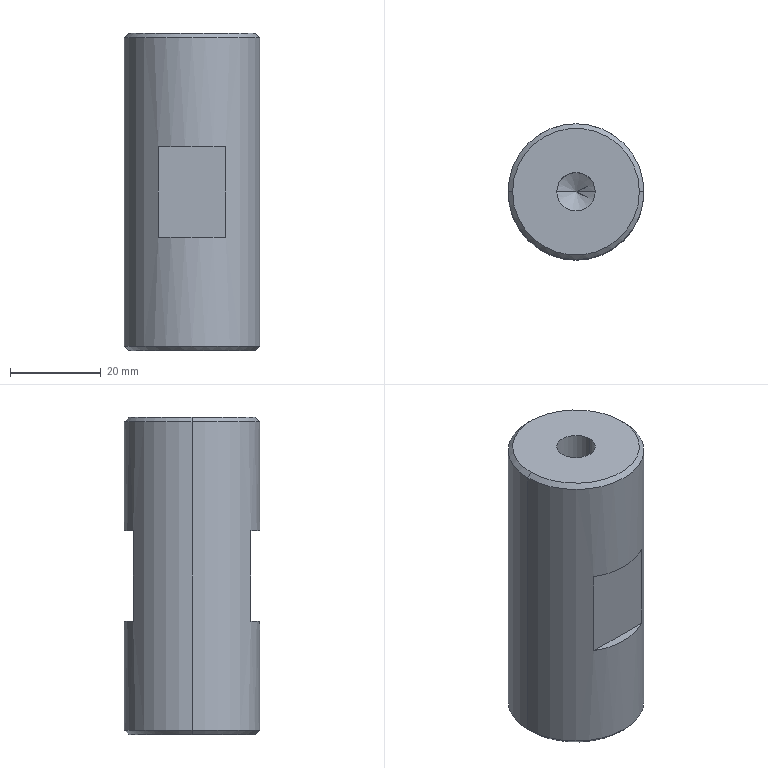Part | STEP file | BB013A02M-04-38A | 1 solid | 22 faces | box 30 x 30 x 70 mm | volume 45701 mm3 | cone 8 | plane 8 | cylinder 6 | commonest cylinder face diameters 8.5 x4 30 x2
STEP:
#1=CARTESIAN_POINT('',(0.,0.,0.));
#2=DIRECTION('',(0.,0.,1.));
#3=DIRECTION('',(1.,0.,0.));
#4=AXIS2_PLACEMENT_3D('',#1,#2,#3);
#5=CARTESIAN_POINT('',(7.483,13.,25.));
#6=VERTEX_POINT('',#5);
#7=CARTESIAN_POINT('',(7.483,13.,45.));
#8=VERTEX_POINT('',#7);
#9=CARTESIAN_POINT('',(7.483,13.,70.));
#10=DIRECTION('',(0.,0.,1.));
#11=VECTOR('',#10,1.);
#12=LINE('',#9,#11);
#13=CARTESIAN_POINT('',(0.,0.,70.));
#14=DIRECTION('',(0.,0.,-1.));
#15=DIRECTION('',(-1.,0.,0.));
#16=AXIS2_PLACEMENT_3D('',#13,#14,#15);
#17=CYLINDRICAL_SURFACE('',#16,15.);
#18=CARTESIAN_POINT('',(2.093,0.));
#19=DIRECTION('',(0.,-1.));
#20=VECTOR('',#19,1.);
#21=LINE('',#18,#20);
#22=(GEOMETRIC_REPRESENTATION_CONTEXT(2)PARAMETRIC_REPRESENTATION_CONTEXT()REPRESENTATION_CONTEXT('',''));
#23=DEFINITIONAL_REPRESENTATION('',(#21),#22);
#24=PCURVE('',#17,#23);
#25=CARTESIAN_POINT('',(7.483,13.,25.));
#26=DIRECTION('',(0.,1.,0.));
#27=DIRECTION('',(-1.,0.,0.));
#28=AXIS2_PLACEMENT_3D('',#25,#26,#27);
#29=PLANE('',#28);
#30=CARTESIAN_POINT('',(0.,45.));
#31=DIRECTION('',(0.,1.));
#32=VECTOR('',#31,1.);
#33=LINE('',#30,#32);
#34=(GEOMETRIC_REPRESENTATION_CONTEXT(2)PARAMETRIC_REPRESENTATION_CONTEXT()REPRESENTATION_CONTEXT('',''));
#35=DEFINITIONAL_REPRESENTATION('',(#33),#34);
#36=PCURVE('',#29,#35);
#37=SURFACE_CURVE('',#12,(#24,#36),.PCURVE_S1.);
#38=EDGE_CURVE('',#6,#8,#37,.T.);
#39=ORIENTED_EDGE('',*,*,#38,.T.);
#40=CARTESIAN_POINT('',(-7.483,13.,45.));
#41=VERTEX_POINT('',#40);
#42=CARTESIAN_POINT('',(0.,0.,45.));
#43=DIRECTION('',(0.,0.,1.));
#44=DIRECTION('',(-1.,0.,0.));
#45=AXIS2_PLACEMENT_3D('',#42,#43,#44);
#46=CIRCLE('',#45,15.);
#47=CARTESIAN_POINT('',(6.283,25.));
#48=DIRECTION('',(-1.,0.));
#49=VECTOR('',#48,1.);
#50=LINE('',#47,#49);
#51=(GEOMETRIC_REPRESENTATION_CONTEXT(2)PARAMETRIC_REPRESENTATION_CONTEXT()REPRESENTATION_CONTEXT('',''));
#52=DEFINITIONAL_REPRESENTATION('',(#50),#51);
#53=PCURVE('',#17,#52);
#54=CARTESIAN_POINT('',(0.,0.,45.));
#55=DIRECTION('',(0.,0.,-1.));
#56=DIRECTION('',(-1.,0.,0.));
#57=AXIS2_PLACEMENT_3D('',#54,#55,#56);
#58=PLANE('',#57);
#59=CARTESIAN_POINT('',(15.,0.));
#60=CARTESIAN_POINT('',(15.,-25.981));
#61=CARTESIAN_POINT('',(-7.5,-12.99));
#62=CARTESIAN_POINT('',(-30.,0.));
#63=CARTESIAN_POINT('',(-7.5,12.99));
#64=CARTESIAN_POINT('',(15.,25.981));
#65=CARTESIAN_POINT('',(15.,0.));
#66=(BOUNDED_CURVE()B_SPLINE_CURVE(2,(#59,#60,#61,#62,#63,#64,#65),.UNSPECIFIED.,.T.,.F.)B_SPLINE_CURVE_WITH_KNOTS((1,2,2,2,2,1),(-2.094,0.,2.094,4.189,6.283,8.378),.UNSPECIFIED.)CURVE()GEOMETRIC_REPRESENTATION_ITEM()RATIONAL_B_SPLINE_CURVE((1.,0.5,1.,0.5,1.,0.5,1.))REPRESENTATION_ITEM(''));
#67=(GEOMETRIC_REPRESENTATION_CONTEXT(2)PARAMETRIC_REPRESENTATION_CONTEXT()REPRESENTATION_CONTEXT('',''));
#68=DEFINITIONAL_REPRESENTATION('',(#66),#67);
#69=PCURVE('',#58,#68);
#70=SURFACE_CURVE('',#46,(#53,#69),.PCURVE_S1.);
#71=EDGE_CURVE('',#8,#41,#70,.T.);
#72=ORIENTED_EDGE('',*,*,#71,.T.);
#73=CARTESIAN_POINT('',(-7.483,13.,25.));
#74=VERTEX_POINT('',#73);
#75=CARTESIAN_POINT('',(-7.483,13.,70.));
#76=DIRECTION('',(0.,0.,-1.));
#77=VECTOR('',#76,1.);
#78=LINE('',#75,#77);
#79=CARTESIAN_POINT('',(1.048,0.));
#80=DIRECTION('',(0.,1.));
#81=VECTOR('',#80,1.);
#82=LINE('',#79,#81);
#83=(GEOMETRIC_REPRESENTATION_CONTEXT(2)PARAMETRIC_REPRESENTATION_CONTEXT()REPRESENTATION_CONTEXT('',''));
#84=DEFINITIONAL_REPRESENTATION('',(#82),#83);
#85=PCURVE('',#17,#84);
#86=CARTESIAN_POINT('',(14.967,45.));
#87=DIRECTION('',(0.,-1.));
#88=VECTOR('',#87,1.);
#89=LINE('',#86,#88);
#90=(GEOMETRIC_REPRESENTATION_CONTEXT(2)PARAMETRIC_REPRESENTATION_CONTEXT()REPRESENTATION_CONTEXT('',''));
#91=DEFINITIONAL_REPRESENTATION('',(#89),#90);
#92=PCURVE('',#29,#91);
#93=SURFACE_CURVE('',#78,(#85,#92),.PCURVE_S1.);
#94=EDGE_CURVE('',#41,#74,#93,.T.);
#95=ORIENTED_EDGE('',*,*,#94,.T.);
#96=CARTESIAN_POINT('',(0.,0.,25.));
#97=DIRECTION('',(0.,0.,-1.));
#98=DIRECTION('',(-1.,0.,0.));
#99=AXIS2_PLACEMENT_3D('',#96,#97,#98);
#100=CIRCLE('',#99,15.);
#101=CARTESIAN_POINT('',(0.,45.));
#102=DIRECTION('',(1.,0.));
#103=VECTOR('',#102,1.);
#104=LINE('',#101,#103);
#105=(GEOMETRIC_REPRESENTATION_CONTEXT(2)PARAMETRIC_REPRESENTATION_CONTEXT()REPRESENTATION_CONTEXT('',''));
#106=DEFINITIONAL_REPRESENTATION('',(#104),#105);
#107=PCURVE('',#17,#106);
#108=CARTESIAN_POINT('',(0.,0.,25.));
#109=DIRECTION('',(0.,0.,-1.));
#110=DIRECTION('',(-1.,0.,0.));
#111=AXIS2_PLACEMENT_3D('',#108,#109,#110);
#112=PLANE('',#111);
#113=CARTESIAN_POINT('',(0.,0.));
#114=DIRECTION('',(1.,0.));
#115=AXIS2_PLACEMENT_2D('',#113,#114);
#116=CIRCLE('',#115,15.);
#117=(GEOMETRIC_REPRESENTATION_CONTEXT(2)PARAMETRIC_REPRESENTATION_CONTEXT()REPRESENTATION_CONTEXT('',''));
#118=DEFINITIONAL_REPRESENTATION('',(#116),#117);
#119=PCURVE('',#112,#118);
#120=SURFACE_CURVE('',#100,(#107,#119),.PCURVE_S1.);
#121=EDGE_CURVE('',#74,#6,#120,.T.);
#122=ORIENTED_EDGE('',*,*,#121,.T.);
#123=EDGE_LOOP('',(#39,#72,#95,#122));
#124=FACE_BOUND('',#123,.T.);
#125=CARTESIAN_POINT('',(-15.,0.,69.));
#126=VERTEX_POINT('',#125);
#127=CARTESIAN_POINT('',(15.,0.,69.));
#128=VERTEX_POINT('',#127);
#129=CARTESIAN_POINT('',(0.,0.,69.));
#130=DIRECTION('',(0.,0.,-1.));
#131=DIRECTION('',(-1.,0.,0.));
#132=AXIS2_PLACEMENT_3D('',#129,#130,#131);
#133=CIRCLE('',#132,15.);
#134=CARTESIAN_POINT('',(0.,1.));
#135=DIRECTION('',(1.,0.));
#136=VECTOR('',#135,1.);
#137=LINE('',#134,#136);
#138=(GEOMETRIC_REPRESENTATION_CONTEXT(2)PARAMETRIC_REPRESENTATION_CONTEXT()REPRESENTATION_CONTEXT('',''));
#139=DEFINITIONAL_REPRESENTATION('',(#137),#138);
#140=PCURVE('',#17,#139);
#141=CARTESIAN_POINT('',(0.,0.,69.));
#142=DIRECTION('',(0.,0.,-1.));
#143=DIRECTION('',(-1.,0.,0.));
#144=AXIS2_PLACEMENT_3D('',#141,#142,#143);
#145=CONICAL_SURFACE('',#144,15.,0.7854);
#146=CARTESIAN_POINT('',(0.,0.));
#147=DIRECTION('',(1.,0.));
#148=VECTOR('',#147,1.);
#149=LINE('',#146,#148);
#150=(GEOMETRIC_REPRESENTATION_CONTEXT(2)PARAMETRIC_REPRESENTATION_CONTEXT()REPRESENTATION_CONTEXT('',''));
#151=DEFINITIONAL_REPRESENTATION('',(#149),#150);
#152=PCURVE('',#145,#151);
#153=SURFACE_CURVE('',#133,(#140,#152),.PCURVE_S1.);
#154=EDGE_CURVE('',#126,#128,#153,.T.);
#155=ORIENTED_EDGE('',*,*,#154,.T.);
#156=CARTESIAN_POINT('',(15.,0.,1.));
#157=VERTEX_POINT('',#156);
#158=CARTESIAN_POINT('',(15.,0.,70.));
#159=DIRECTION('',(0.,0.,-1.));
#160=VECTOR('',#159,1.);
#161=LINE('',#158,#160);
#162=CARTESIAN_POINT('',(3.142,0.));
#163=DIRECTION('',(0.,1.));
#164=VECTOR('',#163,1.);
#165=LINE('',#162,#164);
#166=(GEOMETRIC_REPRESENTATION_CONTEXT(2)PARAMETRIC_REPRESENTATION_CONTEXT()REPRESENTATION_CONTEXT('',''));
#167=DEFINITIONAL_REPRESENTATION('',(#165),#166);
#168=PCURVE('',#17,#167);
#169=CARTESIAN_POINT('',(0.,0.,70.));
#170=DIRECTION('',(0.,0.,-1.));
#171=DIRECTION('',(-1.,0.,0.));
#172=AXIS2_PLACEMENT_3D('',#169,#170,#171);
#173=CYLINDRICAL_SURFACE('',#172,15.);
#174=CARTESIAN_POINT('',(3.142,0.));
#175=DIRECTION('',(0.,1.));
#176=VECTOR('',#175,1.);
#177=LINE('',#174,#176);
#178=(GEOMETRIC_REPRESENTATION_CONTEXT(2)PARAMETRIC_REPRESENTATION_CONTEXT()REPRESENTATION_CONTEXT('',''));
#179=DEFINITIONAL_REPRESENTATION('',(#177),#178);
#180=PCURVE('',#173,#179);
#181=SURFACE_CURVE('',#161,(#168,#180),.PCURVE_S1.);
#182=EDGE_CURVE('',#128,#157,#181,.T.);
#183=ORIENTED_EDGE('',*,*,#182,.T.);
#184=CARTESIAN_POINT('',(-15.,0.,1.));
#185=VERTEX_POINT('',#184);
#186=CARTESIAN_POINT('',(0.,0.,1.));
#187=DIRECTION('',(0.,0.,1.));
#188=DIRECTION('',(-1.,0.,0.));
#189=AXIS2_PLACEMENT_3D('',#186,#187,#188);
#190=CIRCLE('',#189,15.);
#191=CARTESIAN_POINT('',(6.283,69.));
#192=DIRECTION('',(-1.,0.));
#193=VECTOR('',#192,1.);
#194=LINE('',#191,#193);
#195=(GEOMETRIC_REPRESENTATION_CONTEXT(2)PARAMETRIC_REPRESENTATION_CONTEXT()REPRESENTATION_CONTEXT('',''));
#196=DEFINITIONAL_REPRESENTATION('',(#194),#195);
#197=PCURVE('',#17,#196);
#198=CARTESIAN_POINT('',(0.,0.,1.));
#199=DIRECTION('',(0.,0.,1.));
#200=DIRECTION('',(1.,0.,0.));
#201=AXIS2_PLACEMENT_3D('',#198,#199,#200);
#202=CONICAL_SURFACE('',#201,15.,0.7854);
#203=CARTESIAN_POINT('',(-3.142,0.));
#204=DIRECTION('',(1.,0.));
#205=VECTOR('',#204,1.);
#206=LINE('',#203,#205);
#207=(GEOMETRIC_REPRESENTATION_CONTEXT(2)PARAMETRIC_REPRESENTATION_CONTEXT()REPRESENTATION_CONTEXT('',''));
#208=DEFINITIONAL_REPRESENTATION('',(#206),#207);
#209=PCURVE('',#202,#208);
#210=SURFACE_CURVE('',#190,(#197,#209),.PCURVE_S1.);
#211=EDGE_CURVE('',#157,#185,#210,.T.);
#212=ORIENTED_EDGE('',*,*,#211,.T.);
#213=CARTESIAN_POINT('',(-15.,0.,70.));
#214=DIRECTION('',(0.,0.,-1.));
#215=VECTOR('',#214,1.);
#216=LINE('',#213,#215);
#217=CARTESIAN_POINT('',(0.,0.));
#218=DIRECTION('',(0.,1.));
#219=VECTOR('',#218,1.);
#220=LINE('',#217,#219);
#221=(GEOMETRIC_REPRESENTATION_CONTEXT(2)PARAMETRIC_REPRESENTATION_CONTEXT()REPRESENTATION_CONTEXT('',''));
#222=DEFINITIONAL_REPRESENTATION('',(#220),#221);
#223=PCURVE('',#17,#222);
#224=CARTESIAN_POINT('',(6.283,0.));
#225=DIRECTION('',(0.,1.));
#226=VECTOR('',#225,1.);
#227=LINE('',#224,#226);
#228=(GEOMETRIC_REPRESENTATION_CONTEXT(2)PARAMETRIC_REPRESENTATION_CONTEXT()REPRESENTATION_CONTEXT('',''));
#229=DEFINITIONAL_REPRESENTATION('',(#227),#228);
#230=PCURVE('',#173,#229);
#231=SURFACE_CURVE('',#216,(#223,#230),.PCURVE_S1.);
#232=EDGE_CURVE('',#126,#185,#231,.T.);
#233=ORIENTED_EDGE('',*,*,#232,.F.);
#234=EDGE_LOOP('',(#155,#183,#212,#233));
#235=FACE_BOUND('',#234,.T.);
#236=ADVANCED_FACE('',(#124,#235),#17,.T.);
#237=CARTESIAN_POINT('',(14.,0.,0.));
#238=VERTEX_POINT('',#237);
#239=CARTESIAN_POINT('',(-14.,0.,0.));
#240=VERTEX_POINT('',#239);
#241=CARTESIAN_POINT('',(0.,0.,0.));
#242=DIRECTION('',(0.,0.,1.));
#243=DIRECTION('',(1.,0.,0.));
#244=AXIS2_PLACEMENT_3D('',#241,#242,#243);
#245=CIRCLE('',#244,14.);
#246=CARTESIAN_POINT('',(0.,-1.));
#247=DIRECTION('',(1.,0.));
#248=VECTOR('',#247,1.);
#249=LINE('',#246,#248);
#250=(GEOMETRIC_REPRESENTATION_CONTEXT(2)PARAMETRIC_REPRESENTATION_CONTEXT()REPRESENTATION_CONTEXT('',''));
#251=DEFINITIONAL_REPRESENTATION('',(#249),#250);
#252=PCURVE('',#202,#251);
#253=CARTESIAN_POINT('',(0.,0.,0.));
#254=DIRECTION('',(0.,0.,1.));
#255=DIRECTION('',(1.,0.,0.));
#256=AXIS2_PLACEMENT_3D('',#253,#254,#255);
#257=PLANE('',#256);
#258=CARTESIAN_POINT('',(0.,0.));
#259=DIRECTION('',(1.,0.));
#260=AXIS2_PLACEMENT_2D('',#258,#259);
#261=CIRCLE('',#260,14.);
#262=(GEOMETRIC_REPRESENTATION_CONTEXT(2)PARAMETRIC_REPRESENTATION_CONTEXT()REPRESENTATION_CONTEXT('',''));
#263=DEFINITIONAL_REPRESENTATION('',(#261),#262);
#264=PCURVE('',#257,#263);
#265=SURFACE_CURVE('',#245,(#252,#264),.PCURVE_S1.);
#266=EDGE_CURVE('',#238,#240,#265,.T.);
#267=ORIENTED_EDGE('',*,*,#266,.T.);
#268=CARTESIAN_POINT('',(-15.,0.,1.));
#269=DIRECTION('',(-0.7071,0.,0.7071));
#270=VECTOR('',#269,1.);
#271=LINE('',#268,#270);
#272=CARTESIAN_POINT('',(3.142,0.));
#273=DIRECTION('',(0.,1.));
#274=VECTOR('',#273,1.);
#275=LINE('',#272,#274);
#276=(GEOMETRIC_REPRESENTATION_CONTEXT(2)PARAMETRIC_REPRESENTATION_CONTEXT()REPRESENTATION_CONTEXT('',''));
#277=DEFINITIONAL_REPRESENTATION('',(#275),#276);
#278=PCURVE('',#202,#277);
#279=CARTESIAN_POINT('',(0.,0.,1.));
#280=DIRECTION('',(0.,0.,1.));
#281=DIRECTION('',(1.,0.,0.));
#282=AXIS2_PLACEMENT_3D('',#279,#280,#281);
#283=CONICAL_SURFACE('',#282,15.,0.7854);
#284=CARTESIAN_POINT('',(3.142,0.));
#285=DIRECTION('',(0.,1.));
#286=VECTOR('',#285,1.);
#287=LINE('',#284,#286);
#288=(GEOMETRIC_REPRESENTATION_CONTEXT(2)PARAMETRIC_REPRESENTATION_CONTEXT()REPRESENTATION_CONTEXT('',''));
#289=DEFINITIONAL_REPRESENTATION('',(#287),#288);
#290=PCURVE('',#283,#289);
#291=SURFACE_CURVE('',#271,(#278,#290),.PCURVE_S1.);
#292=EDGE_CURVE('',#240,#185,#291,.T.);
#293=ORIENTED_EDGE('',*,*,#292,.T.);
#294=ORIENTED_EDGE('',*,*,#211,.F.);
#295=CARTESIAN_POINT('',(15.,0.,1.));
#296=DIRECTION('',(0.7071,0.,0.7071));
#297=VECTOR('',#296,1.);
#298=LINE('',#295,#297);
#299=CARTESIAN_POINT('',(0.,0.));
#300=DIRECTION('',(0.,1.));
#301=VECTOR('',#300,1.);
#302=LINE('',#299,#301);
#303=(GEOMETRIC_REPRESENTATION_CONTEXT(2)PARAMETRIC_REPRESENTATION_CONTEXT()REPRESENTATION_CONTEXT('',''));
#304=DEFINITIONAL_REPRESENTATION('',(#302),#303);
#305=PCURVE('',#202,#304);
#306=CARTESIAN_POINT('',(6.283,0.));
#307=DIRECTION('',(0.,1.));
#308=VECTOR('',#307,1.);
#309=LINE('',#306,#308);
#310=(GEOMETRIC_REPRESENTATION_CONTEXT(2)PARAMETRIC_REPRESENTATION_CONTEXT()REPRESENTATION_CONTEXT('',''));
#311=DEFINITIONAL_REPRESENTATION('',(#309),#310);
#312=PCURVE('',#283,#311);
#313=SURFACE_CURVE('',#298,(#305,#312),.PCURVE_S1.);
#314=EDGE_CURVE('',#238,#157,#313,.T.);
#315=ORIENTED_EDGE('',*,*,#314,.F.);
#316=EDGE_LOOP('',(#267,#293,#294,#315));
#317=FACE_BOUND('',#316,.T.);
#318=ADVANCED_FACE('',(#317),#202,.T.);
#319=CARTESIAN_POINT('',(-14.,0.,70.));
#320=VERTEX_POINT('',#319);
#321=CARTESIAN_POINT('',(14.,0.,70.));
#322=VERTEX_POINT('',#321);
#323=CARTESIAN_POINT('',(0.,0.,70.));
#324=DIRECTION('',(0.,0.,-1.));
#325=DIRECTION('',(-1.,0.,0.));
#326=AXIS2_PLACEMENT_3D('',#323,#324,#325);
#327=CIRCLE('',#326,14.);
#328=CARTESIAN_POINT('',(0.,-1.));
#329=DIRECTION('',(1.,0.));
#330=VECTOR('',#329,1.);
#331=LINE('',#328,#330);
#332=(GEOMETRIC_REPRESENTATION_CONTEXT(2)PARAMETRIC_REPRESENTATION_CONTEXT()REPRESENTATION_CONTEXT('',''));
#333=DEFINITIONAL_REPRESENTATION('',(#331),#332);
#334=PCURVE('',#145,#333);
#335=CARTESIAN_POINT('',(0.,0.,70.));
#336=DIRECTION('',(0.,0.,1.));
#337=DIRECTION('',(1.,0.,0.));
#338=AXIS2_PLACEMENT_3D('',#335,#336,#337);
#339=PLANE('',#338);
#340=CARTESIAN_POINT('',(-14.,0.));
#341=CARTESIAN_POINT('',(-14.,24.249));
#342=CARTESIAN_POINT('',(7.,12.124));
#343=CARTESIAN_POINT('',(28.,0.));
#344=CARTESIAN_POINT('',(7.,-12.124));
#345=CARTESIAN_POINT('',(-14.,-24.249));
#346=CARTESIAN_POINT('',(-14.,0.));
#347=(BOUNDED_CURVE()B_SPLINE_CURVE(2,(#340,#341,#342,#343,#344,#345,#346),.UNSPECIFIED.,.T.,.F.)B_SPLINE_CURVE_WITH_KNOTS((1,2,2,2,2,1),(-2.094,0.,2.094,4.189,6.283,8.378),.UNSPECIFIED.)CURVE()GEOMETRIC_REPRESENTATION_ITEM()RATIONAL_B_SPLINE_CURVE((1.,0.5,1.,0.5,1.,0.5,1.))REPRESENTATION_ITEM(''));
#348=(GEOMETRIC_REPRESENTATION_CONTEXT(2)PARAMETRIC_REPRESENTATION_CONTEXT()REPRESENTATION_CONTEXT('',''));
#349=DEFINITIONAL_REPRESENTATION('',(#347),#348);
#350=PCURVE('',#339,#349);
#351=SURFACE_CURVE('',#327,(#334,#350),.PCURVE_S1.);
#352=EDGE_CURVE('',#320,#322,#351,.T.);
#353=ORIENTED_EDGE('',*,*,#352,.T.);
#354=CARTESIAN_POINT('',(15.,0.,69.));
#355=DIRECTION('',(0.7071,0.,-0.7071));
#356=VECTOR('',#355,1.);
#357=LINE('',#354,#356);
#358=CARTESIAN_POINT('',(3.142,0.));
#359=DIRECTION('',(0.,1.));
#360=VECTOR('',#359,1.);
#361=LINE('',#358,#360);
#362=(GEOMETRIC_REPRESENTATION_CONTEXT(2)PARAMETRIC_REPRESENTATION_CONTEXT()REPRESENTATION_CONTEXT('',''));
#363=DEFINITIONAL_REPRESENTATION('',(#361),#362);
#364=PCURVE('',#145,#363);
#365=CARTESIAN_POINT('',(0.,0.,69.));
#366=DIRECTION('',(0.,0.,-1.));
#367=DIRECTION('',(-1.,0.,0.));
#368=AXIS2_PLACEMENT_3D('',#365,#366,#367);
#369=CONICAL_SURFACE('',#368,15.,0.7854);
#370=CARTESIAN_POINT('',(3.142,0.));
#371=DIRECTION('',(0.,1.));
#372=VECTOR('',#371,1.);
#373=LINE('',#370,#372);
#374=(GEOMETRIC_REPRESENTATION_CONTEXT(2)PARAMETRIC_REPRESENTATION_CONTEXT()REPRESENTATION_CONTEXT('',''));
#375=DEFINITIONAL_REPRESENTATION('',(#373),#374);
#376=PCURVE('',#369,#375);
#377=SURFACE_CURVE('',#357,(#364,#376),.PCURVE_S1.);
#378=EDGE_CURVE('',#322,#128,#377,.T.);
#379=ORIENTED_EDGE('',*,*,#378,.T.);
#380=ORIENTED_EDGE('',*,*,#154,.F.);
#381=CARTESIAN_POINT('',(-15.,0.,69.));
#382=DIRECTION('',(-0.7071,0.,-0.7071));
#383=VECTOR('',#382,1.);
#384=LINE('',#381,#383);
#385=CARTESIAN_POINT('',(0.,0.));
#386=DIRECTION('',(0.,1.));
#387=VECTOR('',#386,1.);
#388=LINE('',#385,#387);
#389=(GEOMETRIC_REPRESENTATION_CONTEXT(2)PARAMETRIC_REPRESENTATION_CONTEXT()REPRESENTATION_CONTEXT('',''));
#390=DEFINITIONAL_REPRESENTATION('',(#388),#389);
#391=PCURVE('',#145,#390);
#392=CARTESIAN_POINT('',(6.283,0.));
#393=DIRECTION('',(0.,1.));
#394=VECTOR('',#393,1.);
#395=LINE('',#392,#394);
#396=(GEOMETRIC_REPRESENTATION_CONTEXT(2)PARAMETRIC_REPRESENTATION_CONTEXT()REPRESENTATION_CONTEXT('',''));
#397=DEFINITIONAL_REPRESENTATION('',(#395),#396);
#398=PCURVE('',#369,#397);
#399=SURFACE_CURVE('',#384,(#391,#398),.PCURVE_S1.);
#400=EDGE_CURVE('',#320,#126,#399,.T.);
#401=ORIENTED_EDGE('',*,*,#400,.F.);
#402=EDGE_LOOP('',(#353,#379,#380,#401));
#403=FACE_BOUND('',#402,.T.);
#404=ADVANCED_FACE('',(#403),#145,.T.);
#405=CARTESIAN_POINT('',(-4.25,0.,24.5));
#406=VERTEX_POINT('',#405);
#407=CARTESIAN_POINT('',(-4.25,0.,0.));
#408=VERTEX_POINT('',#407);
#409=CARTESIAN_POINT('',(-4.25,0.,0.));
#410=DIRECTION('',(0.,0.,-1.));
#411=VECTOR('',#410,1.);
#412=LINE('',#409,#411);
#413=CARTESIAN_POINT('',(0.,0.,0.));
#414=DIRECTION('',(0.,0.,-1.));
#415=DIRECTION('',(-1.,0.,0.));
#416=AXIS2_PLACEMENT_3D('',#413,#414,#415);
#417=CYLINDRICAL_SURFACE('',#416,4.25);
#418=CARTESIAN_POINT('',(6.283,0.));
#419=DIRECTION('',(0.,1.));
#420=VECTOR('',#419,1.);
#421=LINE('',#418,#420);
#422=(GEOMETRIC_REPRESENTATION_CONTEXT(2)PARAMETRIC_REPRESENTATION_CONTEXT()REPRESENTATION_CONTEXT('',''));
#423=DEFINITIONAL_REPRESENTATION('',(#421),#422);
#424=PCURVE('',#417,#423);
#425=CARTESIAN_POINT('',(0.,0.,0.));
#426=DIRECTION('',(0.,0.,-1.));
#427=DIRECTION('',(-1.,0.,0.));
#428=AXIS2_PLACEMENT_3D('',#425,#426,#427);
#429=CYLINDRICAL_SURFACE('',#428,4.25);
#430=CARTESIAN_POINT('',(0.,0.));
#431=DIRECTION('',(0.,1.));
#432=VECTOR('',#431,1.);
#433=LINE('',#430,#432);
#434=(GEOMETRIC_REPRESENTATION_CONTEXT(2)PARAMETRIC_REPRESENTATION_CONTEXT()REPRESENTATION_CONTEXT('',''));
#435=DEFINITIONAL_REPRESENTATION('',(#433),#434);
#436=PCURVE('',#429,#435);
#437=SURFACE_CURVE('',#412,(#424,#436),.PCURVE_S1.);
#438=EDGE_CURVE('',#406,#408,#437,.T.);
#439=ORIENTED_EDGE('',*,*,#438,.T.);
#440=CARTESIAN_POINT('',(4.25,0.,0.));
#441=VERTEX_POINT('',#440);
#442=CARTESIAN_POINT('',(0.,0.,0.));
#443=DIRECTION('',(0.,0.,-1.));
#444=DIRECTION('',(-1.,0.,0.));
#445=AXIS2_PLACEMENT_3D('',#442,#443,#444);
#446=CIRCLE('',#445,4.25);
#447=CARTESIAN_POINT('',(0.,0.));
#448=DIRECTION('',(1.,0.));
#449=VECTOR('',#448,1.);
#450=LINE('',#447,#449);
#451=(GEOMETRIC_REPRESENTATION_CONTEXT(2)PARAMETRIC_REPRESENTATION_CONTEXT()REPRESENTATION_CONTEXT('',''));
#452=DEFINITIONAL_REPRESENTATION('',(#450),#451);
#453=PCURVE('',#417,#452);
#454=CARTESIAN_POINT('',(-4.25,0.));
#455=CARTESIAN_POINT('',(-4.25,7.361));
#456=CARTESIAN_POINT('',(2.125,3.681));
#457=CARTESIAN_POINT('',(8.5,0.));
#458=CARTESIAN_POINT('',(2.125,-3.681));
#459=CARTESIAN_POINT('',(-4.25,-7.361));
#460=CARTESIAN_POINT('',(-4.25,0.));
#461=(BOUNDED_CURVE()B_SPLINE_CURVE(2,(#454,#455,#456,#457,#458,#459,#460),.UNSPECIFIED.,.T.,.F.)B_SPLINE_CURVE_WITH_KNOTS((1,2,2,2,2,1),(-2.094,0.,2.094,4.189,6.283,8.378),.UNSPECIFIED.)CURVE()GEOMETRIC_REPRESENTATION_ITEM()RATIONAL_B_SPLINE_CURVE((1.,0.5,1.,0.5,1.,0.5,1.))REPRESENTATION_ITEM(''));
#462=(GEOMETRIC_REPRESENTATION_CONTEXT(2)PARAMETRIC_REPRESENTATION_CONTEXT()REPRESENTATION_CONTEXT('',''));
#463=DEFINITIONAL_REPRESENTATION('',(#461),#462);
#464=PCURVE('',#257,#463);
#465=SURFACE_CURVE('',#446,(#453,#464),.PCURVE_S1.);
#466=EDGE_CURVE('',#441,#408,#465,.T.);
#467=ORIENTED_EDGE('',*,*,#466,.F.);
#468=CARTESIAN_POINT('',(4.25,0.,24.5));
#469=VERTEX_POINT('',#468);
#470=CARTESIAN_POINT('',(4.25,0.,0.));
#471=DIRECTION('',(0.,0.,-1.));
#472=VECTOR('',#471,1.);
#473=LINE('',#470,#472);
#474=CARTESIAN_POINT('',(3.142,0.));
#475=DIRECTION('',(0.,1.));
#476=VECTOR('',#475,1.);
#477=LINE('',#474,#476);
#478=(GEOMETRIC_REPRESENTATION_CONTEXT(2)PARAMETRIC_REPRESENTATION_CONTEXT()REPRESENTATION_CONTEXT('',''));
#479=DEFINITIONAL_REPRESENTATION('',(#477),#478);
#480=PCURVE('',#417,#479);
#481=CARTESIAN_POINT('',(3.142,0.));
#482=DIRECTION('',(0.,1.));
#483=VECTOR('',#482,1.);
#484=LINE('',#481,#483);
#485=(GEOMETRIC_REPRESENTATION_CONTEXT(2)PARAMETRIC_REPRESENTATION_CONTEXT()REPRESENTATION_CONTEXT('',''));
#486=DEFINITIONAL_REPRESENTATION('',(#484),#485);
#487=PCURVE('',#429,#486);
#488=SURFACE_CURVE('',#473,(#480,#487),.PCURVE_S1.);
#489=EDGE_CURVE('',#469,#441,#488,.T.);
#490=ORIENTED_EDGE('',*,*,#489,.F.);
#491=CARTESIAN_POINT('',(0.,0.,24.5));
#492=DIRECTION('',(0.,0.,-1.));
#493=DIRECTION('',(-1.,0.,0.));
#494=AXIS2_PLACEMENT_3D('',#491,#492,#493);
#495=CIRCLE('',#494,4.25);
#496=CARTESIAN_POINT('',(0.,-24.5));
#497=DIRECTION('',(1.,0.));
#498=VECTOR('',#497,1.);
#499=LINE('',#496,#498);
#500=(GEOMETRIC_REPRESENTATION_CONTEXT(2)PARAMETRIC_REPRESENTATION_CONTEXT()REPRESENTATION_CONTEXT('',''));
#501=DEFINITIONAL_REPRESENTATION('',(#499),#500);
#502=PCURVE('',#417,#501);
#503=CARTESIAN_POINT('',(0.,0.,24.5));
#504=DIRECTION('',(0.,0.,-1.));
#505=DIRECTION('',(-1.,0.,0.));
#506=AXIS2_PLACEMENT_3D('',#503,#504,#505);
#507=CONICAL_SURFACE('',#506,4.25,1.03);
#508=CARTESIAN_POINT('',(0.,0.));
#509=DIRECTION('',(1.,0.));
#510=VECTOR('',#509,1.);
#511=LINE('',#508,#510);
#512=(GEOMETRIC_REPRESENTATION_CONTEXT(2)PARAMETRIC_REPRESENTATION_CONTEXT()REPRESENTATION_CONTEXT('',''));
#513=DEFINITIONAL_REPRESENTATION('',(#511),#512);
#514=PCURVE('',#507,#513);
#515=SURFACE_CURVE('',#495,(#502,#514),.PCURVE_S1.);
#516=EDGE_CURVE('',#469,#406,#515,.T.);
#517=ORIENTED_EDGE('',*,*,#516,.T.);
#518=EDGE_LOOP('',(#439,#467,#490,#517));
#519=FACE_BOUND('',#518,.F.);
#520=ADVANCED_FACE('',(#519),#417,.F.);
#521=CARTESIAN_POINT('',(4.25,0.,45.5));
#522=VERTEX_POINT('',#521);
#523=CARTESIAN_POINT('',(4.25,0.,70.));
#524=VERTEX_POINT('',#523);
#525=CARTESIAN_POINT('',(4.25,0.,70.));
#526=DIRECTION('',(0.,0.,1.));
#527=VECTOR('',#526,1.);
#528=LINE('',#525,#527);
#529=CARTESIAN_POINT('',(0.,0.,70.));
#530=DIRECTION('',(0.,0.,1.));
#531=DIRECTION('',(1.,0.,0.));
#532=AXIS2_PLACEMENT_3D('',#529,#530,#531);
#533=CYLINDRICAL_SURFACE('',#532,4.25);
#534=CARTESIAN_POINT('',(6.283,0.));
#535=DIRECTION('',(0.,1.));
#536=VECTOR('',#535,1.);
#537=LINE('',#534,#536);
#538=(GEOMETRIC_REPRESENTATION_CONTEXT(2)PARAMETRIC_REPRESENTATION_CONTEXT()REPRESENTATION_CONTEXT('',''));
#539=DEFINITIONAL_REPRESENTATION('',(#537),#538);
#540=PCURVE('',#533,#539);
#541=CARTESIAN_POINT('',(0.,0.,70.));
#542=DIRECTION('',(0.,0.,1.));
#543=DIRECTION('',(1.,0.,0.));
#544=AXIS2_PLACEMENT_3D('',#541,#542,#543);
#545=CYLINDRICAL_SURFACE('',#544,4.25);
#546=CARTESIAN_POINT('',(0.,0.));
#547=DIRECTION('',(0.,1.));
#548=VECTOR('',#547,1.);
#549=LINE('',#546,#548);
#550=(GEOMETRIC_REPRESENTATION_CONTEXT(2)PARAMETRIC_REPRESENTATION_CONTEXT()REPRESENTATION_CONTEXT('',''));
#551=DEFINITIONAL_REPRESENTATION('',(#549),#550);
#552=PCURVE('',#545,#551);
#553=SURFACE_CURVE('',#528,(#540,#552),.PCURVE_S1.);
#554=EDGE_CURVE('',#522,#524,#553,.T.);
#555=ORIENTED_EDGE('',*,*,#554,.T.);
#556=CARTESIAN_POINT('',(-4.25,0.,70.));
#557=VERTEX_POINT('',#556);
#558=CARTESIAN_POINT('',(0.,0.,70.));
#559=DIRECTION('',(0.,0.,-1.));
#560=DIRECTION('',(1.,0.,0.));
#561=AXIS2_PLACEMENT_3D('',#558,#559,#560);
#562=CIRCLE('',#561,4.25);
#563=CARTESIAN_POINT('',(6.283,0.));
#564=DIRECTION('',(-1.,0.));
#565=VECTOR('',#564,1.);
#566=LINE('',#563,#565);
#567=(GEOMETRIC_REPRESENTATION_CONTEXT(2)PARAMETRIC_REPRESENTATION_CONTEXT()REPRESENTATION_CONTEXT('',''));
#568=DEFINITIONAL_REPRESENTATION('',(#566),#567);
#569=PCURVE('',#533,#568);
#570=CARTESIAN_POINT('',(4.25,0.));
#571=CARTESIAN_POINT('',(4.25,-7.361));
#572=CARTESIAN_POINT('',(-2.125,-3.681));
#573=CARTESIAN_POINT('',(-8.5,0.));
#574=CARTESIAN_POINT('',(-2.125,3.681));
#575=CARTESIAN_POINT('',(4.25,7.361));
#576=CARTESIAN_POINT('',(4.25,0.));
#577=(BOUNDED_CURVE()B_SPLINE_CURVE(2,(#570,#571,#572,#573,#574,#575,#576),.UNSPECIFIED.,.T.,.F.)B_SPLINE_CURVE_WITH_KNOTS((1,2,2,2,2,1),(-2.094,0.,2.094,4.189,6.283,8.378),.UNSPECIFIED.)CURVE()GEOMETRIC_REPRESENTATION_ITEM()RATIONAL_B_SPLINE_CURVE((1.,0.5,1.,0.5,1.,0.5,1.))REPRESENTATION_ITEM(''));
#578=(GEOMETRIC_REPRESENTATION_CONTEXT(2)PARAMETRIC_REPRESENTATION_CONTEXT()REPRESENTATION_CONTEXT('',''));
#579=DEFINITIONAL_REPRESENTATION('',(#577),#578);
#580=PCURVE('',#339,#579);
#581=SURFACE_CURVE('',#562,(#569,#580),.PCURVE_S1.);
#582=EDGE_CURVE('',#524,#557,#581,.T.);
#583=ORIENTED_EDGE('',*,*,#582,.T.);
#584=CARTESIAN_POINT('',(-4.25,0.,45.5));
#585=VERTEX_POINT('',#584);
#586=CARTESIAN_POINT('',(-4.25,0.,70.));
#587=DIRECTION('',(0.,0.,1.));
#588=VECTOR('',#587,1.);
#589=LINE('',#586,#588);
#590=CARTESIAN_POINT('',(3.142,0.));
#591=DIRECTION('',(0.,1.));
#592=VECTOR('',#591,1.);
#593=LINE('',#590,#592);
#594=(GEOMETRIC_REPRESENTATION_CONTEXT(2)PARAMETRIC_REPRESENTATION_CONTEXT()REPRESENTATION_CONTEXT('',''));
#595=DEFINITIONAL_REPRESENTATION('',(#593),#594);
#596=PCURVE('',#533,#595);
#597=CARTESIAN_POINT('',(3.142,0.));
#598=DIRECTION('',(0.,1.));
#599=VECTOR('',#598,1.);
#600=LINE('',#597,#599);
#601=(GEOMETRIC_REPRESENTATION_CONTEXT(2)PARAMETRIC_REPRESENTATION_CONTEXT()REPRESENTATION_CONTEXT('',''));
#602=DEFINITIONAL_REPRESENTATION('',(#600),#601);
#603=PCURVE('',#545,#602);
#604=SURFACE_CURVE('',#589,(#596,#603),.PCURVE_S1.);
#605=EDGE_CURVE('',#585,#557,#604,.T.);
#606=ORIENTED_EDGE('',*,*,#605,.F.);
#607=CARTESIAN_POINT('',(0.,0.,45.5));
#608=DIRECTION('',(0.,0.,1.));
#609=DIRECTION('',(1.,0.,0.));
#610=AXIS2_PLACEMENT_3D('',#607,#608,#609);
#611=CIRCLE('',#610,4.25);
#612=CARTESIAN_POINT('',(0.,-24.5));
#613=DIRECTION('',(1.,0.));
#614=VECTOR('',#613,1.);
#615=LINE('',#612,#614);
#616=(GEOMETRIC_REPRESENTATION_CONTEXT(2)PARAMETRIC_REPRESENTATION_CONTEXT()REPRESENTATION_CONTEXT('',''));
#617=DEFINITIONAL_REPRESENTATION('',(#615),#616);
#618=PCURVE('',#533,#617);
#619=CARTESIAN_POINT('',(0.,0.,45.5));
#620=DIRECTION('',(0.,0.,1.));
#621=DIRECTION('',(1.,0.,0.));
#622=AXIS2_PLACEMENT_3D('',#619,#620,#621);
#623=CONICAL_SURFACE('',#622,4.25,1.03);
#624=CARTESIAN_POINT('',(0.,0.));
#625=DIRECTION('',(1.,0.));
#626=VECTOR('',#625,1.);
#627=LINE('',#624,#626);
#628=(GEOMETRIC_REPRESENTATION_CONTEXT(2)PARAMETRIC_REPRESENTATION_CONTEXT()REPRESENTATION_CONTEXT('',''));
#629=DEFINITIONAL_REPRESENTATION('',(#627),#628);
#630=PCURVE('',#623,#629);
#631=SURFACE_CURVE('',#611,(#618,#630),.PCURVE_S1.);
#632=EDGE_CURVE('',#585,#522,#631,.T.);
#633=ORIENTED_EDGE('',*,*,#632,.T.);
#634=EDGE_LOOP('',(#555,#583,#606,#633));
#635=FACE_BOUND('',#634,.F.);
#636=ADVANCED_FACE('',(#635),#533,.F.);
#637=ORIENTED_EDGE('',*,*,#516,.F.);
#638=CARTESIAN_POINT('',(0.,0.,27.054));
#639=VERTEX_POINT('',#638);
#640=CARTESIAN_POINT('',(4.25,0.,24.5));
#641=DIRECTION('',(0.8572,0.,-0.515));
#642=VECTOR('',#641,1.);
#643=LINE('',#640,#642);
#644=CARTESIAN_POINT('',(3.142,0.));
#645=DIRECTION('',(0.,1.));
#646=VECTOR('',#645,1.);
#647=LINE('',#644,#646);
#648=(GEOMETRIC_REPRESENTATION_CONTEXT(2)PARAMETRIC_REPRESENTATION_CONTEXT()REPRESENTATION_CONTEXT('',''));
#649=DEFINITIONAL_REPRESENTATION('',(#647),#648);
#650=PCURVE('',#507,#649);
#651=CARTESIAN_POINT('',(0.,0.,24.5));
#652=DIRECTION('',(0.,0.,-1.));
#653=DIRECTION('',(-1.,0.,0.));
#654=AXIS2_PLACEMENT_3D('',#651,#652,#653);
#655=CONICAL_SURFACE('',#654,4.25,1.03);
#656=CARTESIAN_POINT('',(3.142,0.));
#657=DIRECTION('',(0.,1.));
#658=VECTOR('',#657,1.);
#659=LINE('',#656,#658);
#660=(GEOMETRIC_REPRESENTATION_CONTEXT(2)PARAMETRIC_REPRESENTATION_CONTEXT()REPRESENTATION_CONTEXT('',''));
#661=DEFINITIONAL_REPRESENTATION('',(#659),#660);
#662=PCURVE('',#655,#661);
#663=SURFACE_CURVE('',#643,(#650,#662),.PCURVE_S1.);
#664=EDGE_CURVE('',#639,#469,#663,.T.);
#665=ORIENTED_EDGE('',*,*,#664,.F.);
#666=CARTESIAN_POINT('',(-4.25,0.,24.5));
#667=DIRECTION('',(-0.8572,0.,-0.515));
#668=VECTOR('',#667,1.);
#669=LINE('',#666,#668);
#670=CARTESIAN_POINT('',(6.283,0.));
#671=DIRECTION('',(0.,1.));
#672=VECTOR('',#671,1.);
#673=LINE('',#670,#672);
#674=(GEOMETRIC_REPRESENTATION_CONTEXT(2)PARAMETRIC_REPRESENTATION_CONTEXT()REPRESENTATION_CONTEXT('',''));
#675=DEFINITIONAL_REPRESENTATION('',(#673),#674);
#676=PCURVE('',#507,#675);
#677=CARTESIAN_POINT('',(0.,0.));
#678=DIRECTION('',(0.,1.));
#679=VECTOR('',#678,1.);
#680=LINE('',#677,#679);
#681=(GEOMETRIC_REPRESENTATION_CONTEXT(2)PARAMETRIC_REPRESENTATION_CONTEXT()REPRESENTATION_CONTEXT('',''));
#682=DEFINITIONAL_REPRESENTATION('',(#680),#681);
#683=PCURVE('',#655,#682);
#684=SURFACE_CURVE('',#669,(#676,#683),.PCURVE_S1.);
#685=EDGE_CURVE('',#639,#406,#684,.T.);
#686=ORIENTED_EDGE('',*,*,#685,.T.);
#687=EDGE_LOOP('',(#637,#665,#686));
#688=FACE_BOUND('',#687,.F.);
#689=ADVANCED_FACE('',(#688),#507,.F.);
#690=ORIENTED_EDGE('',*,*,#632,.F.);
#691=CARTESIAN_POINT('',(0.,0.,42.946));
#692=VERTEX_POINT('',#691);
#693=CARTESIAN_POINT('',(-4.25,0.,45.5));
#694=DIRECTION('',(-0.8572,0.,0.515));
#695=VECTOR('',#694,1.);
#696=LINE('',#693,#695);
#697=CARTESIAN_POINT('',(3.142,0.));
#698=DIRECTION('',(0.,1.));
#699=VECTOR('',#698,1.);
#700=LINE('',#697,#699);
#701=(GEOMETRIC_REPRESENTATION_CONTEXT(2)PARAMETRIC_REPRESENTATION_CONTEXT()REPRESENTATION_CONTEXT('',''));
#702=DEFINITIONAL_REPRESENTATION('',(#700),#701);
#703=PCURVE('',#623,#702);
#704=CARTESIAN_POINT('',(0.,0.,45.5));
#705=DIRECTION('',(0.,0.,1.));
#706=DIRECTION('',(1.,0.,0.));
#707=AXIS2_PLACEMENT_3D('',#704,#705,#706);
#708=CONICAL_SURFACE('',#707,4.25,1.03);
#709=CARTESIAN_POINT('',(3.142,0.));
#710=DIRECTION('',(0.,1.));
#711=VECTOR('',#710,1.);
#712=LINE('',#709,#711);
#713=(GEOMETRIC_REPRESENTATION_CONTEXT(2)PARAMETRIC_REPRESENTATION_CONTEXT()REPRESENTATION_CONTEXT('',''));
#714=DEFINITIONAL_REPRESENTATION('',(#712),#713);
#715=PCURVE('',#708,#714);
#716=SURFACE_CURVE('',#696,(#703,#715),.PCURVE_S1.);
#717=EDGE_CURVE('',#692,#585,#716,.T.);
#718=ORIENTED_EDGE('',*,*,#717,.F.);
#719=CARTESIAN_POINT('',(4.25,0.,45.5));
#720=DIRECTION('',(0.8572,0.,0.515));
#721=VECTOR('',#720,1.);
#722=LINE('',#719,#721);
#723=CARTESIAN_POINT('',(6.283,0.));
#724=DIRECTION('',(0.,1.));
#725=VECTOR('',#724,1.);
#726=LINE('',#723,#725);
#727=(GEOMETRIC_REPRESENTATION_CONTEXT(2)PARAMETRIC_REPRESENTATION_CONTEXT()REPRESENTATION_CONTEXT('',''));
#728=DEFINITIONAL_REPRESENTATION('',(#726),#727);
#729=PCURVE('',#623,#728);
#730=CARTESIAN_POINT('',(0.,0.));
#731=DIRECTION('',(0.,1.));
#732=VECTOR('',#731,1.);
#733=LINE('',#730,#732);
#734=(GEOMETRIC_REPRESENTATION_CONTEXT(2)PARAMETRIC_REPRESENTATION_CONTEXT()REPRESENTATION_CONTEXT('',''));
#735=DEFINITIONAL_REPRESENTATION('',(#733),#734);
#736=PCURVE('',#708,#735);
#737=SURFACE_CURVE('',#722,(#729,#736),.PCURVE_S1.);
#738=EDGE_CURVE('',#692,#522,#737,.T.);
#739=ORIENTED_EDGE('',*,*,#738,.T.);
#740=EDGE_LOOP('',(#690,#718,#739));
#741=FACE_BOUND('',#740,.F.);
#742=ADVANCED_FACE('',(#741),#623,.F.);
#743=ORIENTED_EDGE('',*,*,#182,.F.);
#744=CARTESIAN_POINT('',(0.,0.,69.));
#745=DIRECTION('',(0.,0.,-1.));
#746=DIRECTION('',(-1.,0.,0.));
#747=AXIS2_PLACEMENT_3D('',#744,#745,#746);
#748=CIRCLE('',#747,15.);
#749=CARTESIAN_POINT('',(0.,1.));
#750=DIRECTION('',(1.,0.));
#751=VECTOR('',#750,1.);
#752=LINE('',#749,#751);
#753=(GEOMETRIC_REPRESENTATION_CONTEXT(2)PARAMETRIC_REPRESENTATION_CONTEXT()REPRESENTATION_CONTEXT('',''));
#754=DEFINITIONAL_REPRESENTATION('',(#752),#753);
#755=PCURVE('',#173,#754);
#756=CARTESIAN_POINT('',(0.,0.));
#757=DIRECTION('',(1.,0.));
#758=VECTOR('',#757,1.);
#759=LINE('',#756,#758);
#760=(GEOMETRIC_REPRESENTATION_CONTEXT(2)PARAMETRIC_REPRESENTATION_CONTEXT()REPRESENTATION_CONTEXT('',''));
#761=DEFINITIONAL_REPRESENTATION('',(#759),#760);
#762=PCURVE('',#369,#761);
#763=SURFACE_CURVE('',#748,(#755,#762),.PCURVE_S1.);
#764=EDGE_CURVE('',#128,#126,#763,.T.);
#765=ORIENTED_EDGE('',*,*,#764,.T.);
#766=ORIENTED_EDGE('',*,*,#232,.T.);
#767=CARTESIAN_POINT('',(0.,0.,1.));
#768=DIRECTION('',(0.,0.,1.));
#769=DIRECTION('',(-1.,0.,0.));
#770=AXIS2_PLACEMENT_3D('',#767,#768,#769);
#771=CIRCLE('',#770,15.);
#772=CARTESIAN_POINT('',(6.283,69.));
#773=DIRECTION('',(-1.,0.));
#774=VECTOR('',#773,1.);
#775=LINE('',#772,#774);
#776=(GEOMETRIC_REPRESENTATION_CONTEXT(2)PARAMETRIC_REPRESENTATION_CONTEXT()REPRESENTATION_CONTEXT('',''));
#777=DEFINITIONAL_REPRESENTATION('',(#775),#776);
#778=PCURVE('',#173,#777);
#779=CARTESIAN_POINT('',(3.142,0.));
#780=DIRECTION('',(1.,0.));
#781=VECTOR('',#780,1.);
#782=LINE('',#779,#781);
#783=(GEOMETRIC_REPRESENTATION_CONTEXT(2)PARAMETRIC_REPRESENTATION_CONTEXT()REPRESENTATION_CONTEXT('',''));
#784=DEFINITIONAL_REPRESENTATION('',(#782),#783);
#785=PCURVE('',#283,#784);
#786=SURFACE_CURVE('',#771,(#778,#785),.PCURVE_S1.);
#787=EDGE_CURVE('',#185,#157,#786,.T.);
#788=ORIENTED_EDGE('',*,*,#787,.T.);
#789=EDGE_LOOP('',(#743,#765,#766,#788));
#790=FACE_BOUND('',#789,.T.);
#791=CARTESIAN_POINT('',(-7.483,-13.,25.));
#792=VERTEX_POINT('',#791);
#793=CARTESIAN_POINT('',(-7.483,-13.,45.));
#794=VERTEX_POINT('',#793);
#795=CARTESIAN_POINT('',(-7.483,-13.,70.));
#796=DIRECTION('',(0.,0.,1.));
#797=VECTOR('',#796,1.);
#798=LINE('',#795,#797);
#799=CARTESIAN_POINT('',(5.235,0.));
#800=DIRECTION('',(0.,-1.));
#801=VECTOR('',#800,1.);
#802=LINE('',#799,#801);
#803=(GEOMETRIC_REPRESENTATION_CONTEXT(2)PARAMETRIC_REPRESENTATION_CONTEXT()REPRESENTATION_CONTEXT('',''));
#804=DEFINITIONAL_REPRESENTATION('',(#802),#803);
#805=PCURVE('',#173,#804);
#806=CARTESIAN_POINT('',(7.483,-13.,25.));
#807=DIRECTION('',(0.,-1.,0.));
#808=DIRECTION('',(0.,0.,-1.));
#809=AXIS2_PLACEMENT_3D('',#806,#807,#808);
#810=PLANE('',#809);
#811=CARTESIAN_POINT('',(-45.,-14.967));
#812=DIRECTION('',(-1.,0.));
#813=VECTOR('',#812,1.);
#814=LINE('',#811,#813);
#815=(GEOMETRIC_REPRESENTATION_CONTEXT(2)PARAMETRIC_REPRESENTATION_CONTEXT()REPRESENTATION_CONTEXT('',''));
#816=DEFINITIONAL_REPRESENTATION('',(#814),#815);
#817=PCURVE('',#810,#816);
#818=SURFACE_CURVE('',#798,(#805,#817),.PCURVE_S1.);
#819=EDGE_CURVE('',#792,#794,#818,.T.);
#820=ORIENTED_EDGE('',*,*,#819,.T.);
#821=CARTESIAN_POINT('',(7.483,-13.,45.));
#822=VERTEX_POINT('',#821);
#823=CARTESIAN_POINT('',(0.,0.,45.));
#824=DIRECTION('',(0.,0.,1.));
#825=DIRECTION('',(-1.,0.,0.));
#826=AXIS2_PLACEMENT_3D('',#823,#824,#825);
#827=CIRCLE('',#826,15.);
#828=CARTESIAN_POINT('',(6.283,25.));
#829=DIRECTION('',(-1.,0.));
#830=VECTOR('',#829,1.);
#831=LINE('',#828,#830);
#832=(GEOMETRIC_REPRESENTATION_CONTEXT(2)PARAMETRIC_REPRESENTATION_CONTEXT()REPRESENTATION_CONTEXT('',''));
#833=DEFINITIONAL_REPRESENTATION('',(#831),#832);
#834=PCURVE('',#173,#833);
#835=CARTESIAN_POINT('',(0.,0.,45.));
#836=DIRECTION('',(0.,0.,-1.));
#837=DIRECTION('',(-1.,0.,0.));
#838=AXIS2_PLACEMENT_3D('',#835,#836,#837);
#839=PLANE('',#838);
#840=CARTESIAN_POINT('',(15.,0.));
#841=CARTESIAN_POINT('',(15.,-25.981));
#842=CARTESIAN_POINT('',(-7.5,-12.99));
#843=CARTESIAN_POINT('',(-30.,0.));
#844=CARTESIAN_POINT('',(-7.5,12.99));
#845=CARTESIAN_POINT('',(15.,25.981));
#846=CARTESIAN_POINT('',(15.,0.));
#847=(BOUNDED_CURVE()B_SPLINE_CURVE(2,(#840,#841,#842,#843,#844,#845,#846),.UNSPECIFIED.,.T.,.F.)B_SPLINE_CURVE_WITH_KNOTS((1,2,2,2,2,1),(-2.094,0.,2.094,4.189,6.283,8.378),.UNSPECIFIED.)CURVE()GEOMETRIC_REPRESENTATION_ITEM()RATIONAL_B_SPLINE_CURVE((1.,0.5,1.,0.5,1.,0.5,1.))REPRESENTATION_ITEM(''));
#848=(GEOMETRIC_REPRESENTATION_CONTEXT(2)PARAMETRIC_REPRESENTATION_CONTEXT()REPRESENTATION_CONTEXT('',''));
#849=DEFINITIONAL_REPRESENTATION('',(#847),#848);
#850=PCURVE('',#839,#849);
#851=SURFACE_CURVE('',#827,(#834,#850),.PCURVE_S1.);
#852=EDGE_CURVE('',#794,#822,#851,.T.);
#853=ORIENTED_EDGE('',*,*,#852,.T.);
#854=CARTESIAN_POINT('',(7.483,-13.,25.));
#855=VERTEX_POINT('',#854);
#856=CARTESIAN_POINT('',(7.483,-13.,70.));
#857=DIRECTION('',(0.,0.,-1.));
#858=VECTOR('',#857,1.);
#859=LINE('',#856,#858);
#860=CARTESIAN_POINT('',(4.19,0.));
#861=DIRECTION('',(0.,1.));
#862=VECTOR('',#861,1.);
#863=LINE('',#860,#862);
#864=(GEOMETRIC_REPRESENTATION_CONTEXT(2)PARAMETRIC_REPRESENTATION_CONTEXT()REPRESENTATION_CONTEXT('',''));
#865=DEFINITIONAL_REPRESENTATION('',(#863),#864);
#866=PCURVE('',#173,#865);
#867=CARTESIAN_POINT('',(-45.,0.));
#868=DIRECTION('',(1.,0.));
#869=VECTOR('',#868,1.);
#870=LINE('',#867,#869);
#871=(GEOMETRIC_REPRESENTATION_CONTEXT(2)PARAMETRIC_REPRESENTATION_CONTEXT()REPRESENTATION_CONTEXT('',''));
#872=DEFINITIONAL_REPRESENTATION('',(#870),#871);
#873=PCURVE('',#810,#872);
#874=SURFACE_CURVE('',#859,(#866,#873),.PCURVE_S1.);
#875=EDGE_CURVE('',#822,#855,#874,.T.);
#876=ORIENTED_EDGE('',*,*,#875,.T.);
#877=CARTESIAN_POINT('',(0.,0.,25.));
#878=DIRECTION('',(0.,0.,-1.));
#879=DIRECTION('',(-1.,0.,0.));
#880=AXIS2_PLACEMENT_3D('',#877,#878,#879);
#881=CIRCLE('',#880,15.);
#882=CARTESIAN_POINT('',(0.,45.));
#883=DIRECTION('',(1.,0.));
#884=VECTOR('',#883,1.);
#885=LINE('',#882,#884);
#886=(GEOMETRIC_REPRESENTATION_CONTEXT(2)PARAMETRIC_REPRESENTATION_CONTEXT()REPRESENTATION_CONTEXT('',''));
#887=DEFINITIONAL_REPRESENTATION('',(#885),#886);
#888=PCURVE('',#173,#887);
#889=CARTESIAN_POINT('',(0.,0.,25.));
#890=DIRECTION('',(0.,0.,-1.));
#891=DIRECTION('',(-1.,0.,0.));
#892=AXIS2_PLACEMENT_3D('',#889,#890,#891);
#893=PLANE('',#892);
#894=CARTESIAN_POINT('',(0.,0.));
#895=DIRECTION('',(1.,0.));
#896=AXIS2_PLACEMENT_2D('',#894,#895);
#897=CIRCLE('',#896,15.);
#898=(GEOMETRIC_REPRESENTATION_CONTEXT(2)PARAMETRIC_REPRESENTATION_CONTEXT()REPRESENTATION_CONTEXT('',''));
#899=DEFINITIONAL_REPRESENTATION('',(#897),#898);
#900=PCURVE('',#893,#899);
#901=SURFACE_CURVE('',#881,(#888,#900),.PCURVE_S1.);
#902=EDGE_CURVE('',#855,#792,#901,.T.);
#903=ORIENTED_EDGE('',*,*,#902,.T.);
#904=EDGE_LOOP('',(#820,#853,#876,#903));
#905=FACE_BOUND('',#904,.T.);
#906=ADVANCED_FACE('',(#790,#905),#173,.T.);
#907=ORIENTED_EDGE('',*,*,#292,.F.);
#908=CARTESIAN_POINT('',(0.,0.,0.));
#909=DIRECTION('',(0.,0.,1.));
#910=DIRECTION('',(1.,0.,0.));
#911=AXIS2_PLACEMENT_3D('',#908,#909,#910);
#912=CIRCLE('',#911,14.);
#913=CARTESIAN_POINT('',(0.,-1.));
#914=DIRECTION('',(1.,0.));
#915=VECTOR('',#914,1.);
#916=LINE('',#913,#915);
#917=(GEOMETRIC_REPRESENTATION_CONTEXT(2)PARAMETRIC_REPRESENTATION_CONTEXT()REPRESENTATION_CONTEXT('',''));
#918=DEFINITIONAL_REPRESENTATION('',(#916),#917);
#919=PCURVE('',#283,#918);
#920=CARTESIAN_POINT('',(0.,0.));
#921=DIRECTION('',(1.,0.));
#922=AXIS2_PLACEMENT_2D('',#920,#921);
#923=CIRCLE('',#922,14.);
#924=(GEOMETRIC_REPRESENTATION_CONTEXT(2)PARAMETRIC_REPRESENTATION_CONTEXT()REPRESENTATION_CONTEXT('',''));
#925=DEFINITIONAL_REPRESENTATION('',(#923),#924);
#926=PCURVE('',#257,#925);
#927=SURFACE_CURVE('',#912,(#919,#926),.PCURVE_S1.);
#928=EDGE_CURVE('',#240,#238,#927,.T.);
#929=ORIENTED_EDGE('',*,*,#928,.T.);
#930=ORIENTED_EDGE('',*,*,#314,.T.);
#931=ORIENTED_EDGE('',*,*,#787,.F.);
#932=EDGE_LOOP('',(#907,#929,#930,#931));
#933=FACE_BOUND('',#932,.T.);
#934=ADVANCED_FACE('',(#933),#283,.T.);
#935=ORIENTED_EDGE('',*,*,#378,.F.);
#936=CARTESIAN_POINT('',(0.,0.,70.));
#937=DIRECTION('',(0.,0.,-1.));
#938=DIRECTION('',(-1.,0.,0.));
#939=AXIS2_PLACEMENT_3D('',#936,#937,#938);
#940=CIRCLE('',#939,14.);
#941=CARTESIAN_POINT('',(0.,-1.));
#942=DIRECTION('',(1.,0.));
#943=VECTOR('',#942,1.);
#944=LINE('',#941,#943);
#945=(GEOMETRIC_REPRESENTATION_CONTEXT(2)PARAMETRIC_REPRESENTATION_CONTEXT()REPRESENTATION_CONTEXT('',''));
#946=DEFINITIONAL_REPRESENTATION('',(#944),#945);
#947=PCURVE('',#369,#946);
#948=CARTESIAN_POINT('',(-14.,0.));
#949=CARTESIAN_POINT('',(-14.,24.249));
#950=CARTESIAN_POINT('',(7.,12.124));
#951=CARTESIAN_POINT('',(28.,0.));
#952=CARTESIAN_POINT('',(7.,-12.124));
#953=CARTESIAN_POINT('',(-14.,-24.249));
#954=CARTESIAN_POINT('',(-14.,0.));
#955=(BOUNDED_CURVE()B_SPLINE_CURVE(2,(#948,#949,#950,#951,#952,#953,#954),.UNSPECIFIED.,.T.,.F.)B_SPLINE_CURVE_WITH_KNOTS((1,2,2,2,2,1),(-2.094,0.,2.094,4.189,6.283,8.378),.UNSPECIFIED.)CURVE()GEOMETRIC_REPRESENTATION_ITEM()RATIONAL_B_SPLINE_CURVE((1.,0.5,1.,0.5,1.,0.5,1.))REPRESENTATION_ITEM(''));
#956=(GEOMETRIC_REPRESENTATION_CONTEXT(2)PARAMETRIC_REPRESENTATION_CONTEXT()REPRESENTATION_CONTEXT('',''));
#957=DEFINITIONAL_REPRESENTATION('',(#955),#956);
#958=PCURVE('',#339,#957);
#959=SURFACE_CURVE('',#940,(#947,#958),.PCURVE_S1.);
#960=EDGE_CURVE('',#322,#320,#959,.T.);
#961=ORIENTED_EDGE('',*,*,#960,.T.);
#962=ORIENTED_EDGE('',*,*,#400,.T.);
#963=ORIENTED_EDGE('',*,*,#764,.F.);
#964=EDGE_LOOP('',(#935,#961,#962,#963));
#965=FACE_BOUND('',#964,.T.);
#966=ADVANCED_FACE('',(#965),#369,.T.);
#967=ORIENTED_EDGE('',*,*,#71,.F.);
#968=CARTESIAN_POINT('',(0.,13.,45.));
#969=DIRECTION('',(-1.,0.,0.));
#970=VECTOR('',#969,1.);
#971=LINE('',#968,#970);
#972=CARTESIAN_POINT('',(0.,13.));
#973=DIRECTION('',(1.,0.));
#974=VECTOR('',#973,1.);
#975=LINE('',#972,#974);
#976=(GEOMETRIC_REPRESENTATION_CONTEXT(2)PARAMETRIC_REPRESENTATION_CONTEXT()REPRESENTATION_CONTEXT('',''));
#977=DEFINITIONAL_REPRESENTATION('',(#975),#976);
#978=PCURVE('',#58,#977);
#979=CARTESIAN_POINT('',(7.483,20.));
#980=DIRECTION('',(1.,0.));
#981=VECTOR('',#980,1.);
#982=LINE('',#979,#981);
#983=(GEOMETRIC_REPRESENTATION_CONTEXT(2)PARAMETRIC_REPRESENTATION_CONTEXT()REPRESENTATION_CONTEXT('',''));
#984=DEFINITIONAL_REPRESENTATION('',(#982),#983);
#985=PCURVE('',#29,#984);
#986=SURFACE_CURVE('',#971,(#978,#985),.PCURVE_S1.);
#987=EDGE_CURVE('',#8,#41,#986,.T.);
#988=ORIENTED_EDGE('',*,*,#987,.T.);
#989=EDGE_LOOP('',(#967,#988));
#990=FACE_BOUND('',#989,.T.);
#991=ADVANCED_FACE('',(#990),#58,.T.);
#992=CARTESIAN_POINT('',(7.483,13.,25.));
#993=DIRECTION('',(-1.,0.,0.));
#994=VECTOR('',#993,1.);
#995=LINE('',#992,#994);
#996=CARTESIAN_POINT('',(0.,0.));
#997=DIRECTION('',(1.,0.));
#998=VECTOR('',#997,1.);
#999=LINE('',#996,#998);
#1000=(GEOMETRIC_REPRESENTATION_CONTEXT(2)PARAMETRIC_REPRESENTATION_CONTEXT()REPRESENTATION_CONTEXT('',''));
#1001=DEFINITIONAL_REPRESENTATION('',(#999),#1000);
#1002=PCURVE('',#29,#1001);
#1003=CARTESIAN_POINT('',(-7.483,13.));
#1004=DIRECTION('',(1.,0.));
#1005=VECTOR('',#1004,1.);
#1006=LINE('',#1003,#1005);
#1007=(GEOMETRIC_REPRESENTATION_CONTEXT(2)PARAMETRIC_REPRESENTATION_CONTEXT()REPRESENTATION_CONTEXT('',''));
#1008=DEFINITIONAL_REPRESENTATION('',(#1006),#1007);
#1009=PCURVE('',#112,#1008);
#1010=SURFACE_CURVE('',#995,(#1002,#1009),.PCURVE_S1.);
#1011=EDGE_CURVE('',#6,#74,#1010,.T.);
#1012=ORIENTED_EDGE('',*,*,#1011,.T.);
#1013=ORIENTED_EDGE('',*,*,#94,.F.);
#1014=ORIENTED_EDGE('',*,*,#987,.F.);
#1015=ORIENTED_EDGE('',*,*,#38,.F.);
#1016=EDGE_LOOP('',(#1012,#1013,#1014,#1015));
#1017=FACE_BOUND('',#1016,.T.);
#1018=ADVANCED_FACE('',(#1017),#29,.T.);
#1019=ORIENTED_EDGE('',*,*,#1011,.F.);
#1020=ORIENTED_EDGE('',*,*,#121,.F.);
#1021=EDGE_LOOP('',(#1019,#1020));
#1022=FACE_BOUND('',#1021,.T.);
#1023=ADVANCED_FACE('',(#1022),#112,.F.);
#1024=ORIENTED_EDGE('',*,*,#852,.F.);
#1025=CARTESIAN_POINT('',(0.,-13.,45.));
#1026=DIRECTION('',(1.,0.,0.));
#1027=VECTOR('',#1026,1.);
#1028=LINE('',#1025,#1027);
#1029=CARTESIAN_POINT('',(0.,-13.));
#1030=DIRECTION('',(-1.,0.));
#1031=VECTOR('',#1030,1.);
#1032=LINE('',#1029,#1031);
#1033=(GEOMETRIC_REPRESENTATION_CONTEXT(2)PARAMETRIC_REPRESENTATION_CONTEXT()REPRESENTATION_CONTEXT('',''));
#1034=DEFINITIONAL_REPRESENTATION('',(#1032),#1033);
#1035=PCURVE('',#839,#1034);
#1036=CARTESIAN_POINT('',(-20.,-7.483));
#1037=DIRECTION('',(0.,1.));
#1038=VECTOR('',#1037,1.);
#1039=LINE('',#1036,#1038);
#1040=(GEOMETRIC_REPRESENTATION_CONTEXT(2)PARAMETRIC_REPRESENTATION_CONTEXT()REPRESENTATION_CONTEXT('',''));
#1041=DEFINITIONAL_REPRESENTATION('',(#1039),#1040);
#1042=PCURVE('',#810,#1041);
#1043=SURFACE_CURVE('',#1028,(#1035,#1042),.PCURVE_S1.);
#1044=EDGE_CURVE('',#794,#822,#1043,.T.);
#1045=ORIENTED_EDGE('',*,*,#1044,.T.);
#1046=EDGE_LOOP('',(#1024,#1045));
#1047=FACE_BOUND('',#1046,.T.);
#1048=ADVANCED_FACE('',(#1047),#839,.T.);
#1049=CARTESIAN_POINT('',(7.483,-13.,25.));
#1050=DIRECTION('',(1.,0.,0.));
#1051=VECTOR('',#1050,1.);
#1052=LINE('',#1049,#1051);
#1053=CARTESIAN_POINT('',(0.,0.));
#1054=DIRECTION('',(0.,1.));
#1055=VECTOR('',#1054,1.);
#1056=LINE('',#1053,#1055);
#1057=(GEOMETRIC_REPRESENTATION_CONTEXT(2)PARAMETRIC_REPRESENTATION_CONTEXT()REPRESENTATION_CONTEXT('',''));
#1058=DEFINITIONAL_REPRESENTATION('',(#1056),#1057);
#1059=PCURVE('',#810,#1058);
#1060=CARTESIAN_POINT('',(-7.483,-13.));
#1061=DIRECTION('',(-1.,0.));
#1062=VECTOR('',#1061,1.);
#1063=LINE('',#1060,#1062);
#1064=(GEOMETRIC_REPRESENTATION_CONTEXT(2)PARAMETRIC_REPRESENTATION_CONTEXT()REPRESENTATION_CONTEXT('',''));
#1065=DEFINITIONAL_REPRESENTATION('',(#1063),#1064);
#1066=PCURVE('',#893,#1065);
#1067=SURFACE_CURVE('',#1052,(#1059,#1066),.PCURVE_S1.);
#1068=EDGE_CURVE('',#792,#855,#1067,.T.);
#1069=ORIENTED_EDGE('',*,*,#1068,.T.);
#1070=ORIENTED_EDGE('',*,*,#875,.F.);
#1071=ORIENTED_EDGE('',*,*,#1044,.F.);
#1072=ORIENTED_EDGE('',*,*,#819,.F.);
#1073=EDGE_LOOP('',(#1069,#1070,#1071,#1072));
#1074=FACE_BOUND('',#1073,.T.);
#1075=ADVANCED_FACE('',(#1074),#810,.T.);
#1076=ORIENTED_EDGE('',*,*,#1068,.F.);
#1077=ORIENTED_EDGE('',*,*,#902,.F.);
#1078=EDGE_LOOP('',(#1076,#1077));
#1079=FACE_BOUND('',#1078,.T.);
#1080=ADVANCED_FACE('',(#1079),#893,.F.);
#1081=CARTESIAN_POINT('',(0.,0.,0.));
#1082=DIRECTION('',(0.,0.,-1.));
#1083=DIRECTION('',(-1.,0.,0.));
#1084=AXIS2_PLACEMENT_3D('',#1081,#1082,#1083);
#1085=CIRCLE('',#1084,4.25);
#1086=CARTESIAN_POINT('',(-4.25,0.));
#1087=CARTESIAN_POINT('',(-4.25,7.361));
#1088=CARTESIAN_POINT('',(2.125,3.681));
#1089=CARTESIAN_POINT('',(8.5,0.));
#1090=CARTESIAN_POINT('',(2.125,-3.681));
#1091=CARTESIAN_POINT('',(-4.25,-7.361));
#1092=CARTESIAN_POINT('',(-4.25,0.));
#1093=(BOUNDED_CURVE()B_SPLINE_CURVE(2,(#1086,#1087,#1088,#1089,#1090,#1091,#1092),.UNSPECIFIED.,.T.,.F.)B_SPLINE_CURVE_WITH_KNOTS((1,2,2,2,2,1),(-2.094,0.,2.094,4.189,6.283,8.378),.UNSPECIFIED.)CURVE()GEOMETRIC_REPRESENTATION_ITEM()RATIONAL_B_SPLINE_CURVE((1.,0.5,1.,0.5,1.,0.5,1.))REPRESENTATION_ITEM(''));
#1094=(GEOMETRIC_REPRESENTATION_CONTEXT(2)PARAMETRIC_REPRESENTATION_CONTEXT()REPRESENTATION_CONTEXT('',''));
#1095=DEFINITIONAL_REPRESENTATION('',(#1093),#1094);
#1096=PCURVE('',#257,#1095);
#1097=CARTESIAN_POINT('',(0.,0.));
#1098=DIRECTION('',(1.,0.));
#1099=VECTOR('',#1098,1.);
#1100=LINE('',#1097,#1099);
#1101=(GEOMETRIC_REPRESENTATION_CONTEXT(2)PARAMETRIC_REPRESENTATION_CONTEXT()REPRESENTATION_CONTEXT('',''));
#1102=DEFINITIONAL_REPRESENTATION('',(#1100),#1101);
#1103=PCURVE('',#429,#1102);
#1104=SURFACE_CURVE('',#1085,(#1096,#1103),.PCURVE_S1.);
#1105=EDGE_CURVE('',#408,#441,#1104,.T.);
#1106=ORIENTED_EDGE('',*,*,#1105,.F.);
#1107=ORIENTED_EDGE('',*,*,#466,.F.);
#1108=EDGE_LOOP('',(#1106,#1107));
#1109=FACE_BOUND('',#1108,.T.);
#1110=ORIENTED_EDGE('',*,*,#266,.F.);
#1111=ORIENTED_EDGE('',*,*,#928,.F.);
#1112=EDGE_LOOP('',(#1110,#1111));
#1113=FACE_BOUND('',#1112,.T.);
#1114=ADVANCED_FACE('',(#1109,#1113),#257,.F.);
#1115=ORIENTED_EDGE('',*,*,#582,.T.);
#1116=CARTESIAN_POINT('',(0.,0.,70.));
#1117=DIRECTION('',(0.,0.,-1.));
#1118=DIRECTION('',(1.,0.,0.));
#1119=AXIS2_PLACEMENT_3D('',#1116,#1117,#1118);
#1120=CIRCLE('',#1119,4.25);
#1121=CARTESIAN_POINT('',(4.25,0.));
#1122=CARTESIAN_POINT('',(4.25,-7.361));
#1123=CARTESIAN_POINT('',(-2.125,-3.681));
#1124=CARTESIAN_POINT('',(-8.5,0.));
#1125=CARTESIAN_POINT('',(-2.125,3.681));
#1126=CARTESIAN_POINT('',(4.25,7.361));
#1127=CARTESIAN_POINT('',(4.25,0.));
#1128=(BOUNDED_CURVE()B_SPLINE_CURVE(2,(#1121,#1122,#1123,#1124,#1125,#1126,#1127),.UNSPECIFIED.,.T.,.F.)B_SPLINE_CURVE_WITH_KNOTS((1,2,2,2,2,1),(-2.094,0.,2.094,4.189,6.283,8.378),.UNSPECIFIED.)CURVE()GEOMETRIC_REPRESENTATION_ITEM()RATIONAL_B_SPLINE_CURVE((1.,0.5,1.,0.5,1.,0.5,1.))REPRESENTATION_ITEM(''));
#1129=(GEOMETRIC_REPRESENTATION_CONTEXT(2)PARAMETRIC_REPRESENTATION_CONTEXT()REPRESENTATION_CONTEXT('',''));
#1130=DEFINITIONAL_REPRESENTATION('',(#1128),#1129);
#1131=PCURVE('',#339,#1130);
#1132=CARTESIAN_POINT('',(6.283,0.));
#1133=DIRECTION('',(-1.,0.));
#1134=VECTOR('',#1133,1.);
#1135=LINE('',#1132,#1134);
#1136=(GEOMETRIC_REPRESENTATION_CONTEXT(2)PARAMETRIC_REPRESENTATION_CONTEXT()REPRESENTATION_CONTEXT('',''));
#1137=DEFINITIONAL_REPRESENTATION('',(#1135),#1136);
#1138=PCURVE('',#545,#1137);
#1139=SURFACE_CURVE('',#1120,(#1131,#1138),.PCURVE_S1.);
#1140=EDGE_CURVE('',#557,#524,#1139,.T.);
#1141=ORIENTED_EDGE('',*,*,#1140,.T.);
#1142=EDGE_LOOP('',(#1115,#1141));
#1143=FACE_BOUND('',#1142,.T.);
#1144=ORIENTED_EDGE('',*,*,#352,.F.);
#1145=ORIENTED_EDGE('',*,*,#960,.F.);
#1146=EDGE_LOOP('',(#1144,#1145));
#1147=FACE_BOUND('',#1146,.T.);
#1148=ADVANCED_FACE('',(#1143,#1147),#339,.T.);
#1149=ORIENTED_EDGE('',*,*,#1105,.F.);
#1150=ORIENTED_EDGE('',*,*,#438,.F.);
#1151=CARTESIAN_POINT('',(0.,0.,24.5));
#1152=DIRECTION('',(0.,0.,-1.));
#1153=DIRECTION('',(-1.,0.,0.));
#1154=AXIS2_PLACEMENT_3D('',#1151,#1152,#1153);
#1155=CIRCLE('',#1154,4.25);
#1156=CARTESIAN_POINT('',(0.,-24.5));
#1157=DIRECTION('',(1.,0.));
#1158=VECTOR('',#1157,1.);
#1159=LINE('',#1156,#1158);
#1160=(GEOMETRIC_REPRESENTATION_CONTEXT(2)PARAMETRIC_REPRESENTATION_CONTEXT()REPRESENTATION_CONTEXT('',''));
#1161=DEFINITIONAL_REPRESENTATION('',(#1159),#1160);
#1162=PCURVE('',#429,#1161);
#1163=CARTESIAN_POINT('',(0.,0.));
#1164=DIRECTION('',(1.,0.));
#1165=VECTOR('',#1164,1.);
#1166=LINE('',#1163,#1165);
#1167=(GEOMETRIC_REPRESENTATION_CONTEXT(2)PARAMETRIC_REPRESENTATION_CONTEXT()REPRESENTATION_CONTEXT('',''));
#1168=DEFINITIONAL_REPRESENTATION('',(#1166),#1167);
#1169=PCURVE('',#655,#1168);
#1170=SURFACE_CURVE('',#1155,(#1162,#1169),.PCURVE_S1.);
#1171=EDGE_CURVE('',#406,#469,#1170,.T.);
#1172=ORIENTED_EDGE('',*,*,#1171,.T.);
#1173=ORIENTED_EDGE('',*,*,#489,.T.);
#1174=EDGE_LOOP('',(#1149,#1150,#1172,#1173));
#1175=FACE_BOUND('',#1174,.F.);
#1176=ADVANCED_FACE('',(#1175),#429,.F.);
#1177=ORIENTED_EDGE('',*,*,#1140,.T.);
#1178=ORIENTED_EDGE('',*,*,#554,.F.);
#1179=CARTESIAN_POINT('',(0.,0.,45.5));
#1180=DIRECTION('',(0.,0.,1.));
#1181=DIRECTION('',(1.,0.,0.));
#1182=AXIS2_PLACEMENT_3D('',#1179,#1180,#1181);
#1183=CIRCLE('',#1182,4.25);
#1184=CARTESIAN_POINT('',(0.,-24.5));
#1185=DIRECTION('',(1.,0.));
#1186=VECTOR('',#1185,1.);
#1187=LINE('',#1184,#1186);
#1188=(GEOMETRIC_REPRESENTATION_CONTEXT(2)PARAMETRIC_REPRESENTATION_CONTEXT()REPRESENTATION_CONTEXT('',''));
#1189=DEFINITIONAL_REPRESENTATION('',(#1187),#1188);
#1190=PCURVE('',#545,#1189);
#1191=CARTESIAN_POINT('',(0.,0.));
#1192=DIRECTION('',(1.,0.));
#1193=VECTOR('',#1192,1.);
#1194=LINE('',#1191,#1193);
#1195=(GEOMETRIC_REPRESENTATION_CONTEXT(2)PARAMETRIC_REPRESENTATION_CONTEXT()REPRESENTATION_CONTEXT('',''));
#1196=DEFINITIONAL_REPRESENTATION('',(#1194),#1195);
#1197=PCURVE('',#708,#1196);
#1198=SURFACE_CURVE('',#1183,(#1190,#1197),.PCURVE_S1.);
#1199=EDGE_CURVE('',#522,#585,#1198,.T.);
#1200=ORIENTED_EDGE('',*,*,#1199,.T.);
#1201=ORIENTED_EDGE('',*,*,#605,.T.);
#1202=EDGE_LOOP('',(#1177,#1178,#1200,#1201));
#1203=FACE_BOUND('',#1202,.F.);
#1204=ADVANCED_FACE('',(#1203),#545,.F.);
#1205=ORIENTED_EDGE('',*,*,#1171,.F.);
#1206=ORIENTED_EDGE('',*,*,#685,.F.);
#1207=ORIENTED_EDGE('',*,*,#664,.T.);
#1208=EDGE_LOOP('',(#1205,#1206,#1207));
#1209=FACE_BOUND('',#1208,.F.);
#1210=ADVANCED_FACE('',(#1209),#655,.F.);
#1211=ORIENTED_EDGE('',*,*,#1199,.F.);
#1212=ORIENTED_EDGE('',*,*,#738,.F.);
#1213=ORIENTED_EDGE('',*,*,#717,.T.);
#1214=EDGE_LOOP('',(#1211,#1212,#1213));
#1215=FACE_BOUND('',#1214,.F.);
#1216=ADVANCED_FACE('',(#1215),#708,.F.);
#1217=CLOSED_SHELL('',(#236,#318,#404,#520,#636,#689,#742,#906,#934,#966,#991,#1018,#1023,#1048,#1075,#1080,#1114,#1148,#1176,#1204,#1210,#1216));
#1218=MANIFOLD_SOLID_BREP('',#1217);
#1219=(LENGTH_UNIT()NAMED_UNIT(*)SI_UNIT(.MILLI.,.METRE.));
#1220=UNCERTAINTY_MEASURE_WITH_UNIT(LENGTH_MEASURE(0.0000001),#1219,'','');
#1221=(NAMED_UNIT(*)PLANE_ANGLE_UNIT()SI_UNIT($,.RADIAN.));
#1222=(NAMED_UNIT(*)SI_UNIT($,.STERADIAN.)SOLID_ANGLE_UNIT());
#1223=(GEOMETRIC_REPRESENTATION_CONTEXT(3)GLOBAL_UNCERTAINTY_ASSIGNED_CONTEXT((#1220))GLOBAL_UNIT_ASSIGNED_CONTEXT((#1219,#1221,#1222))REPRESENTATION_CONTEXT('',''));
#1224=ADVANCED_BREP_SHAPE_REPRESENTATION('',(#4,#1218),#1223);